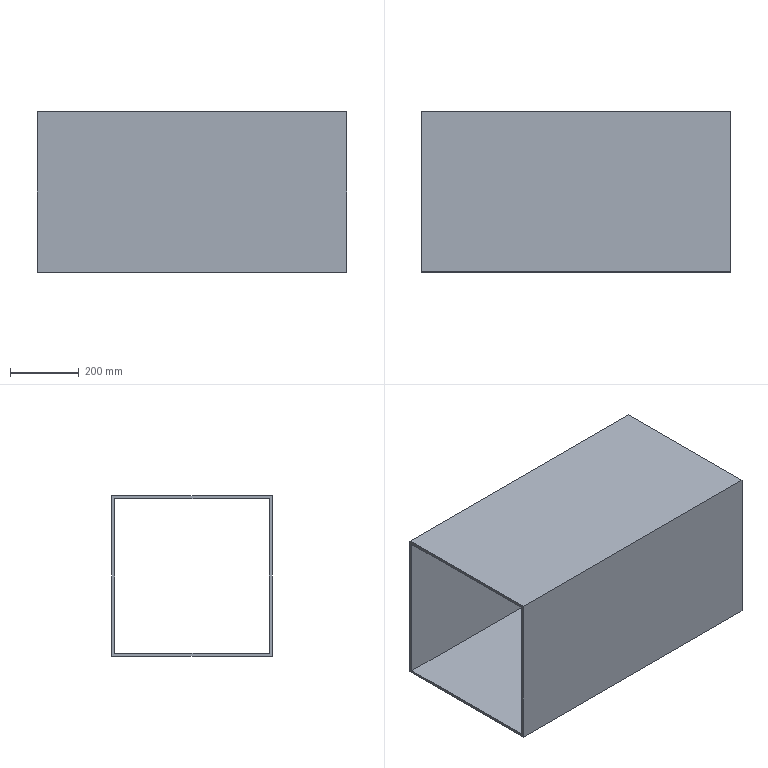Part | SolidWorks | features Extrusion 1 | 1 solid | 10 faces | box 900 x 466 x 466 mm | volume 13190400 mm3 | plane 10
STEP:
#1=CARTESIAN_POINT('',(900.,-233.,-233.));
#2=VERTEX_POINT('',#1);
#3=CARTESIAN_POINT('',(900.,233.,-233.));
#4=VERTEX_POINT('',#3);
#5=CARTESIAN_POINT('',(900.,233.,-233.));
#6=DIRECTION('',(0.,1.,0.));
#7=VECTOR('',#6,1000.);
#8=LINE('',#5,#7);
#9=EDGE_CURVE('',#2,#4,#8,.T.);
#10=ORIENTED_EDGE('',*,*,#9,.T.);
#11=CARTESIAN_POINT('',(900.,233.,233.));
#12=VERTEX_POINT('',#11);
#13=CARTESIAN_POINT('',(900.,233.,233.));
#14=DIRECTION('',(0.,0.,1.));
#15=VECTOR('',#14,1000.);
#16=LINE('',#13,#15);
#17=EDGE_CURVE('',#4,#12,#16,.T.);
#18=ORIENTED_EDGE('',*,*,#17,.T.);
#19=CARTESIAN_POINT('',(900.,-233.,233.));
#20=VERTEX_POINT('',#19);
#21=CARTESIAN_POINT('',(900.,233.,233.));
#22=DIRECTION('',(0.,-1.,0.));
#23=VECTOR('',#22,1000.);
#24=LINE('',#21,#23);
#25=EDGE_CURVE('',#12,#20,#24,.T.);
#26=ORIENTED_EDGE('',*,*,#25,.T.);
#27=CARTESIAN_POINT('',(900.,-233.,233.));
#28=DIRECTION('',(0.,0.,-1.));
#29=VECTOR('',#28,1000.);
#30=LINE('',#27,#29);
#31=EDGE_CURVE('',#20,#2,#30,.T.);
#32=ORIENTED_EDGE('',*,*,#31,.T.);
#33=EDGE_LOOP('',(#10,#18,#26,#32));
#34=FACE_OUTER_BOUND('',#33,.T.);
#35=CARTESIAN_POINT('',(900.,225.,-225.));
#36=VERTEX_POINT('',#35);
#37=CARTESIAN_POINT('',(900.,225.,225.));
#38=VERTEX_POINT('',#37);
#39=CARTESIAN_POINT('',(900.,225.,225.));
#40=DIRECTION('',(0.,0.,1.));
#41=VECTOR('',#40,1000.);
#42=LINE('',#39,#41);
#43=EDGE_CURVE('',#36,#38,#42,.T.);
#44=ORIENTED_EDGE('',*,*,#43,.F.);
#45=CARTESIAN_POINT('',(900.,-225.,-225.));
#46=VERTEX_POINT('',#45);
#47=CARTESIAN_POINT('',(900.,225.,-225.));
#48=DIRECTION('',(0.,1.,0.));
#49=VECTOR('',#48,1000.);
#50=LINE('',#47,#49);
#51=EDGE_CURVE('',#46,#36,#50,.T.);
#52=ORIENTED_EDGE('',*,*,#51,.F.);
#53=CARTESIAN_POINT('',(900.,-225.,225.));
#54=VERTEX_POINT('',#53);
#55=CARTESIAN_POINT('',(900.,-225.,225.));
#56=DIRECTION('',(0.,0.,-1.));
#57=VECTOR('',#56,1000.);
#58=LINE('',#55,#57);
#59=EDGE_CURVE('',#54,#46,#58,.T.);
#60=ORIENTED_EDGE('',*,*,#59,.F.);
#61=CARTESIAN_POINT('',(900.,225.,225.));
#62=DIRECTION('',(0.,-1.,0.));
#63=VECTOR('',#62,1000.);
#64=LINE('',#61,#63);
#65=EDGE_CURVE('',#38,#54,#64,.T.);
#66=ORIENTED_EDGE('',*,*,#65,.F.);
#67=EDGE_LOOP('',(#44,#52,#60,#66));
#68=FACE_BOUND('',#67,.T.);
#69=CARTESIAN_POINT('',(900.,0.,0.));
#70=DIRECTION('',(1.,0.,0.));
#71=DIRECTION('',(0.,0.,-1.));
#72=AXIS2_PLACEMENT_3D('',#69,#70,#71);
#73=PLANE('',#72);
#74=ADVANCED_FACE('',(#34,#68),#73,.T.);
#75=CARTESIAN_POINT('',(0.,-233.,-233.));
#76=VERTEX_POINT('',#75);
#77=CARTESIAN_POINT('',(0.,233.,-233.));
#78=VERTEX_POINT('',#77);
#79=CARTESIAN_POINT('',(0.,233.,-233.));
#80=DIRECTION('',(0.,1.,0.));
#81=VECTOR('',#80,1000.);
#82=LINE('',#79,#81);
#83=EDGE_CURVE('',#76,#78,#82,.T.);
#84=ORIENTED_EDGE('',*,*,#83,.F.);
#85=CARTESIAN_POINT('',(0.,-233.,233.));
#86=VERTEX_POINT('',#85);
#87=CARTESIAN_POINT('',(0.,-233.,233.));
#88=DIRECTION('',(0.,0.,-1.));
#89=VECTOR('',#88,1000.);
#90=LINE('',#87,#89);
#91=EDGE_CURVE('',#86,#76,#90,.T.);
#92=ORIENTED_EDGE('',*,*,#91,.F.);
#93=CARTESIAN_POINT('',(0.,233.,233.));
#94=VERTEX_POINT('',#93);
#95=CARTESIAN_POINT('',(0.,233.,233.));
#96=DIRECTION('',(0.,-1.,0.));
#97=VECTOR('',#96,1000.);
#98=LINE('',#95,#97);
#99=EDGE_CURVE('',#94,#86,#98,.T.);
#100=ORIENTED_EDGE('',*,*,#99,.F.);
#101=CARTESIAN_POINT('',(0.,233.,233.));
#102=DIRECTION('',(0.,0.,1.));
#103=VECTOR('',#102,1000.);
#104=LINE('',#101,#103);
#105=EDGE_CURVE('',#78,#94,#104,.T.);
#106=ORIENTED_EDGE('',*,*,#105,.F.);
#107=EDGE_LOOP('',(#84,#92,#100,#106));
#108=FACE_OUTER_BOUND('',#107,.T.);
#109=CARTESIAN_POINT('',(0.,-225.,-225.));
#110=VERTEX_POINT('',#109);
#111=CARTESIAN_POINT('',(0.,225.,-225.));
#112=VERTEX_POINT('',#111);
#113=CARTESIAN_POINT('',(0.,225.,-225.));
#114=DIRECTION('',(0.,1.,0.));
#115=VECTOR('',#114,1000.);
#116=LINE('',#113,#115);
#117=EDGE_CURVE('',#110,#112,#116,.T.);
#118=ORIENTED_EDGE('',*,*,#117,.T.);
#119=CARTESIAN_POINT('',(0.,225.,225.));
#120=VERTEX_POINT('',#119);
#121=CARTESIAN_POINT('',(0.,225.,225.));
#122=DIRECTION('',(0.,0.,1.));
#123=VECTOR('',#122,1000.);
#124=LINE('',#121,#123);
#125=EDGE_CURVE('',#112,#120,#124,.T.);
#126=ORIENTED_EDGE('',*,*,#125,.T.);
#127=CARTESIAN_POINT('',(0.,-225.,225.));
#128=VERTEX_POINT('',#127);
#129=CARTESIAN_POINT('',(0.,225.,225.));
#130=DIRECTION('',(0.,-1.,0.));
#131=VECTOR('',#130,1000.);
#132=LINE('',#129,#131);
#133=EDGE_CURVE('',#120,#128,#132,.T.);
#134=ORIENTED_EDGE('',*,*,#133,.T.);
#135=CARTESIAN_POINT('',(0.,-225.,225.));
#136=DIRECTION('',(0.,0.,-1.));
#137=VECTOR('',#136,1000.);
#138=LINE('',#135,#137);
#139=EDGE_CURVE('',#128,#110,#138,.T.);
#140=ORIENTED_EDGE('',*,*,#139,.T.);
#141=EDGE_LOOP('',(#118,#126,#134,#140));
#142=FACE_BOUND('',#141,.T.);
#143=CARTESIAN_POINT('',(0.,0.,0.));
#144=DIRECTION('',(1.,0.,0.));
#145=DIRECTION('',(0.,0.,-1.));
#146=AXIS2_PLACEMENT_3D('',#143,#144,#145);
#147=PLANE('',#146);
#148=ADVANCED_FACE('',(#108,#142),#147,.F.);
#149=ORIENTED_EDGE('',*,*,#83,.T.);
#150=CARTESIAN_POINT('',(900.,233.,-233.));
#151=DIRECTION('',(-1.,0.,0.));
#152=VECTOR('',#151,1000.);
#153=LINE('',#150,#152);
#154=EDGE_CURVE('',#4,#78,#153,.T.);
#155=ORIENTED_EDGE('',*,*,#154,.F.);
#156=ORIENTED_EDGE('',*,*,#9,.F.);
#157=CARTESIAN_POINT('',(900.,-233.,-233.));
#158=DIRECTION('',(-1.,0.,0.));
#159=VECTOR('',#158,1000.);
#160=LINE('',#157,#159);
#161=EDGE_CURVE('',#2,#76,#160,.T.);
#162=ORIENTED_EDGE('',*,*,#161,.T.);
#163=EDGE_LOOP('',(#149,#155,#156,#162));
#164=FACE_OUTER_BOUND('',#163,.T.);
#165=CARTESIAN_POINT('',(900.,233.,-233.));
#166=DIRECTION('',(0.,0.,1.));
#167=DIRECTION('',(0.,-1.,0.));
#168=AXIS2_PLACEMENT_3D('',#165,#166,#167);
#169=PLANE('',#168);
#170=ADVANCED_FACE('',(#164),#169,.F.);
#171=ORIENTED_EDGE('',*,*,#105,.T.);
#172=CARTESIAN_POINT('',(900.,233.,233.));
#173=DIRECTION('',(-1.,0.,0.));
#174=VECTOR('',#173,1000.);
#175=LINE('',#172,#174);
#176=EDGE_CURVE('',#12,#94,#175,.T.);
#177=ORIENTED_EDGE('',*,*,#176,.F.);
#178=ORIENTED_EDGE('',*,*,#17,.F.);
#179=ORIENTED_EDGE('',*,*,#154,.T.);
#180=EDGE_LOOP('',(#171,#177,#178,#179));
#181=FACE_OUTER_BOUND('',#180,.T.);
#182=CARTESIAN_POINT('',(900.,233.,233.));
#183=DIRECTION('',(0.,-1.,0.));
#184=DIRECTION('',(0.,0.,-1.));
#185=AXIS2_PLACEMENT_3D('',#182,#183,#184);
#186=PLANE('',#185);
#187=ADVANCED_FACE('',(#181),#186,.F.);
#188=ORIENTED_EDGE('',*,*,#99,.T.);
#189=CARTESIAN_POINT('',(900.,-233.,233.));
#190=DIRECTION('',(-1.,0.,0.));
#191=VECTOR('',#190,1000.);
#192=LINE('',#189,#191);
#193=EDGE_CURVE('',#20,#86,#192,.T.);
#194=ORIENTED_EDGE('',*,*,#193,.F.);
#195=ORIENTED_EDGE('',*,*,#25,.F.);
#196=ORIENTED_EDGE('',*,*,#176,.T.);
#197=EDGE_LOOP('',(#188,#194,#195,#196));
#198=FACE_OUTER_BOUND('',#197,.T.);
#199=CARTESIAN_POINT('',(900.,233.,233.));
#200=DIRECTION('',(0.,0.,-1.));
#201=DIRECTION('',(0.,1.,0.));
#202=AXIS2_PLACEMENT_3D('',#199,#200,#201);
#203=PLANE('',#202);
#204=ADVANCED_FACE('',(#198),#203,.F.);
#205=ORIENTED_EDGE('',*,*,#91,.T.);
#206=ORIENTED_EDGE('',*,*,#161,.F.);
#207=ORIENTED_EDGE('',*,*,#31,.F.);
#208=ORIENTED_EDGE('',*,*,#193,.T.);
#209=EDGE_LOOP('',(#205,#206,#207,#208));
#210=FACE_OUTER_BOUND('',#209,.T.);
#211=CARTESIAN_POINT('',(900.,-233.,233.));
#212=DIRECTION('',(0.,1.,0.));
#213=DIRECTION('',(0.,0.,1.));
#214=AXIS2_PLACEMENT_3D('',#211,#212,#213);
#215=PLANE('',#214);
#216=ADVANCED_FACE('',(#210),#215,.F.);
#217=ORIENTED_EDGE('',*,*,#117,.F.);
#218=CARTESIAN_POINT('',(900.,-225.,-225.));
#219=DIRECTION('',(-1.,0.,0.));
#220=VECTOR('',#219,1000.);
#221=LINE('',#218,#220);
#222=EDGE_CURVE('',#46,#110,#221,.T.);
#223=ORIENTED_EDGE('',*,*,#222,.F.);
#224=ORIENTED_EDGE('',*,*,#51,.T.);
#225=CARTESIAN_POINT('',(900.,225.,-225.));
#226=DIRECTION('',(-1.,0.,0.));
#227=VECTOR('',#226,1000.);
#228=LINE('',#225,#227);
#229=EDGE_CURVE('',#36,#112,#228,.T.);
#230=ORIENTED_EDGE('',*,*,#229,.T.);
#231=EDGE_LOOP('',(#217,#223,#224,#230));
#232=FACE_OUTER_BOUND('',#231,.T.);
#233=CARTESIAN_POINT('',(900.,225.,-225.));
#234=DIRECTION('',(0.,0.,1.));
#235=DIRECTION('',(0.,-1.,0.));
#236=AXIS2_PLACEMENT_3D('',#233,#234,#235);
#237=PLANE('',#236);
#238=ADVANCED_FACE('',(#232),#237,.T.);
#239=ORIENTED_EDGE('',*,*,#125,.F.);
#240=ORIENTED_EDGE('',*,*,#229,.F.);
#241=ORIENTED_EDGE('',*,*,#43,.T.);
#242=CARTESIAN_POINT('',(900.,225.,225.));
#243=DIRECTION('',(-1.,0.,0.));
#244=VECTOR('',#243,1000.);
#245=LINE('',#242,#244);
#246=EDGE_CURVE('',#38,#120,#245,.T.);
#247=ORIENTED_EDGE('',*,*,#246,.T.);
#248=EDGE_LOOP('',(#239,#240,#241,#247));
#249=FACE_OUTER_BOUND('',#248,.T.);
#250=CARTESIAN_POINT('',(900.,225.,225.));
#251=DIRECTION('',(0.,-1.,0.));
#252=DIRECTION('',(0.,0.,-1.));
#253=AXIS2_PLACEMENT_3D('',#250,#251,#252);
#254=PLANE('',#253);
#255=ADVANCED_FACE('',(#249),#254,.T.);
#256=ORIENTED_EDGE('',*,*,#133,.F.);
#257=ORIENTED_EDGE('',*,*,#246,.F.);
#258=ORIENTED_EDGE('',*,*,#65,.T.);
#259=CARTESIAN_POINT('',(900.,-225.,225.));
#260=DIRECTION('',(-1.,0.,0.));
#261=VECTOR('',#260,1000.);
#262=LINE('',#259,#261);
#263=EDGE_CURVE('',#54,#128,#262,.T.);
#264=ORIENTED_EDGE('',*,*,#263,.T.);
#265=EDGE_LOOP('',(#256,#257,#258,#264));
#266=FACE_OUTER_BOUND('',#265,.T.);
#267=CARTESIAN_POINT('',(900.,225.,225.));
#268=DIRECTION('',(0.,0.,-1.));
#269=DIRECTION('',(0.,1.,0.));
#270=AXIS2_PLACEMENT_3D('',#267,#268,#269);
#271=PLANE('',#270);
#272=ADVANCED_FACE('',(#266),#271,.T.);
#273=ORIENTED_EDGE('',*,*,#139,.F.);
#274=ORIENTED_EDGE('',*,*,#263,.F.);
#275=ORIENTED_EDGE('',*,*,#59,.T.);
#276=ORIENTED_EDGE('',*,*,#222,.T.);
#277=EDGE_LOOP('',(#273,#274,#275,#276));
#278=FACE_OUTER_BOUND('',#277,.T.);
#279=CARTESIAN_POINT('',(900.,-225.,225.));
#280=DIRECTION('',(0.,1.,0.));
#281=DIRECTION('',(0.,0.,1.));
#282=AXIS2_PLACEMENT_3D('',#279,#280,#281);
#283=PLANE('',#282);
#284=ADVANCED_FACE('',(#278),#283,.T.);
#285=CLOSED_SHELL('',(#74,#148,#170,#187,#204,#216,#238,#255,#272,#284));
#286=MANIFOLD_SOLID_BREP('',#285);
#287=CARTESIAN_POINT('',(0.,0.,0.));
#288=DIRECTION('',(0.,0.,1.));
#289=DIRECTION('',(1.,0.,0.));
#290=AXIS2_PLACEMENT_3D('',#287,#288,#289);
#291=(LENGTH_UNIT()NAMED_UNIT(*)SI_UNIT(.MILLI.,.METRE.));
#292=UNCERTAINTY_MEASURE_WITH_UNIT(LENGTH_MEASURE(0.00001),#291,'','');
#293=(NAMED_UNIT(*)PLANE_ANGLE_UNIT()SI_UNIT($,.RADIAN.));
#294=(NAMED_UNIT(*)SI_UNIT($,.STERADIAN.)SOLID_ANGLE_UNIT());
#295=(GEOMETRIC_REPRESENTATION_CONTEXT(3)GLOBAL_UNCERTAINTY_ASSIGNED_CONTEXT((#292))GLOBAL_UNIT_ASSIGNED_CONTEXT((#291,#293,#294))REPRESENTATION_CONTEXT('',''));
#296=ADVANCED_BREP_SHAPE_REPRESENTATION('',(#286,#290),#295);